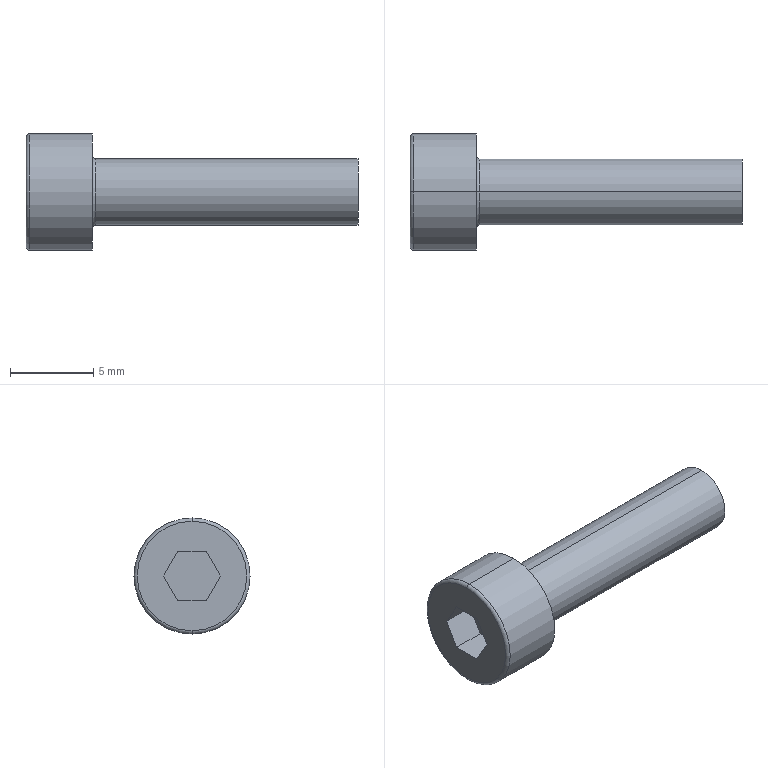Part | SolidWorks | features BlendCut 1, Cut 1, Fillet 1, LPattern 1, RevCut 1, Revolution 1 | 1 solid | 18 faces | box 20 x 7 x 7 mm | volume 339.552 mm3 | plane 10 | torus 4 | cylinder 4 | commonest cylinder face diameters 4 x2 7 x2
STEP:
#1=CARTESIAN_POINT('',(0.2,0.,-3.5));
#2=VERTEX_POINT('',#1);
#3=CARTESIAN_POINT('',(0.2,0.,3.5));
#4=VERTEX_POINT('',#3);
#5=CARTESIAN_POINT('',(0.2,0.,0.));
#6=DIRECTION('',(1.,0.,0.));
#7=DIRECTION('',(0.,0.,1.));
#8=AXIS2_PLACEMENT_3D('',#5,#6,#7);
#9=CIRCLE('',#8,3.5);
#10=EDGE_CURVE('',#2,#4,#9,.T.);
#11=ORIENTED_EDGE('',*,*,#10,.F.);
#12=CARTESIAN_POINT('',(0.,0.,-3.3));
#13=VERTEX_POINT('',#12);
#14=CARTESIAN_POINT('',(0.2,0.,-3.3));
#15=DIRECTION('',(0.,1.,0.));
#16=DIRECTION('',(0.,0.,1.));
#17=AXIS2_PLACEMENT_3D('',#14,#15,#16);
#18=CIRCLE('',#17,0.2);
#19=EDGE_CURVE('',#2,#13,#18,.T.);
#20=ORIENTED_EDGE('',*,*,#19,.T.);
#21=CARTESIAN_POINT('',(0.,0.,3.3));
#22=VERTEX_POINT('',#21);
#23=CARTESIAN_POINT('',(0.,0.,0.));
#24=DIRECTION('',(-1.,0.,0.));
#25=DIRECTION('',(0.,0.,1.));
#26=AXIS2_PLACEMENT_3D('',#23,#24,#25);
#27=CIRCLE('',#26,3.3);
#28=EDGE_CURVE('',#22,#13,#27,.T.);
#29=ORIENTED_EDGE('',*,*,#28,.F.);
#30=CARTESIAN_POINT('',(0.2,0.,3.3));
#31=DIRECTION('',(0.,-1.,0.));
#32=DIRECTION('',(0.,0.,-1.));
#33=AXIS2_PLACEMENT_3D('',#30,#31,#32);
#34=CIRCLE('',#33,0.2);
#35=EDGE_CURVE('',#4,#22,#34,.T.);
#36=ORIENTED_EDGE('',*,*,#35,.F.);
#37=EDGE_LOOP('',(#11,#20,#29,#36));
#38=FACE_OUTER_BOUND('',#37,.T.);
#39=CARTESIAN_POINT('',(0.2,0.,0.));
#40=DIRECTION('',(-1.,0.,0.));
#41=DIRECTION('',(0.,0.,1.));
#42=AXIS2_PLACEMENT_3D('',#39,#40,#41);
#43=TOROIDAL_SURFACE('',#42,3.3,0.2);
#44=ADVANCED_FACE('',(#38),#43,.T.);
#45=CARTESIAN_POINT('',(4.2,0.,-2.));
#46=VERTEX_POINT('',#45);
#47=CARTESIAN_POINT('',(4.2,0.,2.));
#48=VERTEX_POINT('',#47);
#49=CARTESIAN_POINT('',(4.2,0.,0.));
#50=DIRECTION('',(1.,0.,0.));
#51=DIRECTION('',(0.,0.,-1.));
#52=AXIS2_PLACEMENT_3D('',#49,#50,#51);
#53=CIRCLE('',#52,2.);
#54=EDGE_CURVE('',#46,#48,#53,.T.);
#55=ORIENTED_EDGE('',*,*,#54,.T.);
#56=CARTESIAN_POINT('',(20.,0.,2.));
#57=VERTEX_POINT('',#56);
#58=CARTESIAN_POINT('',(0.,0.,2.));
#59=DIRECTION('',(1.,0.,0.));
#60=VECTOR('',#59,1000.);
#61=LINE('',#58,#60);
#62=EDGE_CURVE('',#48,#57,#61,.T.);
#63=ORIENTED_EDGE('',*,*,#62,.T.);
#64=CARTESIAN_POINT('',(20.,0.,-2.));
#65=VERTEX_POINT('',#64);
#66=CARTESIAN_POINT('',(20.,0.,0.));
#67=DIRECTION('',(1.,0.,0.));
#68=DIRECTION('',(0.,0.,-1.));
#69=AXIS2_PLACEMENT_3D('',#66,#67,#68);
#70=CIRCLE('',#69,2.);
#71=EDGE_CURVE('',#65,#57,#70,.T.);
#72=ORIENTED_EDGE('',*,*,#71,.F.);
#73=CARTESIAN_POINT('',(0.,0.,-2.));
#74=DIRECTION('',(1.,0.,0.));
#75=VECTOR('',#74,1000.);
#76=LINE('',#73,#75);
#77=EDGE_CURVE('',#46,#65,#76,.T.);
#78=ORIENTED_EDGE('',*,*,#77,.F.);
#79=EDGE_LOOP('',(#55,#63,#72,#78));
#80=FACE_OUTER_BOUND('',#79,.T.);
#81=CARTESIAN_POINT('',(0.,0.,0.));
#82=DIRECTION('',(1.,0.,0.));
#83=DIRECTION('',(0.,0.,-1.));
#84=AXIS2_PLACEMENT_3D('',#81,#82,#83);
#85=CYLINDRICAL_SURFACE('',#84,2.);
#86=ADVANCED_FACE('',(#80),#85,.T.);
#87=CARTESIAN_POINT('',(4.2,0.,0.));
#88=DIRECTION('',(1.,0.,0.));
#89=DIRECTION('',(0.,0.,-1.));
#90=AXIS2_PLACEMENT_3D('',#87,#88,#89);
#91=CIRCLE('',#90,2.);
#92=EDGE_CURVE('',#48,#46,#91,.T.);
#93=ORIENTED_EDGE('',*,*,#92,.F.);
#94=CARTESIAN_POINT('',(4.,0.,2.2));
#95=VERTEX_POINT('',#94);
#96=CARTESIAN_POINT('',(4.2,0.,2.2));
#97=DIRECTION('',(0.,1.,0.));
#98=DIRECTION('',(0.,0.,1.));
#99=AXIS2_PLACEMENT_3D('',#96,#97,#98);
#100=CIRCLE('',#99,0.2);
#101=EDGE_CURVE('',#48,#95,#100,.T.);
#102=ORIENTED_EDGE('',*,*,#101,.T.);
#103=CARTESIAN_POINT('',(4.,0.,-2.2));
#104=VERTEX_POINT('',#103);
#105=CARTESIAN_POINT('',(4.,0.,0.));
#106=DIRECTION('',(1.,0.,0.));
#107=DIRECTION('',(0.,0.,-1.));
#108=AXIS2_PLACEMENT_3D('',#105,#106,#107);
#109=CIRCLE('',#108,2.2);
#110=EDGE_CURVE('',#95,#104,#109,.T.);
#111=ORIENTED_EDGE('',*,*,#110,.T.);
#112=CARTESIAN_POINT('',(4.2,0.,-2.2));
#113=DIRECTION('',(0.,-1.,0.));
#114=DIRECTION('',(0.,0.,-1.));
#115=AXIS2_PLACEMENT_3D('',#112,#113,#114);
#116=CIRCLE('',#115,0.2);
#117=EDGE_CURVE('',#46,#104,#116,.T.);
#118=ORIENTED_EDGE('',*,*,#117,.F.);
#119=EDGE_LOOP('',(#93,#102,#111,#118));
#120=FACE_OUTER_BOUND('',#119,.T.);
#121=CARTESIAN_POINT('',(4.2,0.,0.));
#122=DIRECTION('',(1.,0.,0.));
#123=DIRECTION('',(0.,0.,-1.));
#124=AXIS2_PLACEMENT_3D('',#121,#122,#123);
#125=TOROIDAL_SURFACE('',#124,2.2,0.2);
#126=ADVANCED_FACE('',(#120),#125,.F.);
#127=ORIENTED_EDGE('',*,*,#10,.T.);
#128=CARTESIAN_POINT('',(4.,0.,3.5));
#129=VERTEX_POINT('',#128);
#130=CARTESIAN_POINT('',(0.,0.,3.5));
#131=DIRECTION('',(1.,0.,0.));
#132=VECTOR('',#131,1000.);
#133=LINE('',#130,#132);
#134=EDGE_CURVE('',#4,#129,#133,.T.);
#135=ORIENTED_EDGE('',*,*,#134,.T.);
#136=CARTESIAN_POINT('',(4.,0.,-3.5));
#137=VERTEX_POINT('',#136);
#138=CARTESIAN_POINT('',(4.,0.,0.));
#139=DIRECTION('',(1.,0.,0.));
#140=DIRECTION('',(0.,0.,-1.));
#141=AXIS2_PLACEMENT_3D('',#138,#139,#140);
#142=CIRCLE('',#141,3.5);
#143=EDGE_CURVE('',#137,#129,#142,.T.);
#144=ORIENTED_EDGE('',*,*,#143,.F.);
#145=CARTESIAN_POINT('',(0.,0.,-3.5));
#146=DIRECTION('',(1.,0.,0.));
#147=VECTOR('',#146,1000.);
#148=LINE('',#145,#147);
#149=EDGE_CURVE('',#2,#137,#148,.T.);
#150=ORIENTED_EDGE('',*,*,#149,.F.);
#151=EDGE_LOOP('',(#127,#135,#144,#150));
#152=FACE_OUTER_BOUND('',#151,.T.);
#153=CARTESIAN_POINT('',(0.,0.,0.));
#154=DIRECTION('',(1.,0.,0.));
#155=DIRECTION('',(0.,0.,-1.));
#156=AXIS2_PLACEMENT_3D('',#153,#154,#155);
#157=CYLINDRICAL_SURFACE('',#156,3.5);
#158=ADVANCED_FACE('',(#152),#157,.T.);
#159=ORIENTED_EDGE('',*,*,#28,.T.);
#160=CARTESIAN_POINT('',(0.,0.,0.));
#161=DIRECTION('',(-1.,0.,0.));
#162=DIRECTION('',(0.,0.,1.));
#163=AXIS2_PLACEMENT_3D('',#160,#161,#162);
#164=CIRCLE('',#163,3.3);
#165=EDGE_CURVE('',#13,#22,#164,.T.);
#166=ORIENTED_EDGE('',*,*,#165,.T.);
#167=EDGE_LOOP('',(#159,#166));
#168=FACE_OUTER_BOUND('',#167,.T.);
#169=CARTESIAN_POINT('',(0.,-1.72,0.));
#170=VERTEX_POINT('',#169);
#171=CARTESIAN_POINT('',(0.,-0.86,1.49));
#172=VERTEX_POINT('',#171);
#173=CARTESIAN_POINT('',(0.,-1.72,0.));
#174=DIRECTION('',(0.,0.5,0.866));
#175=VECTOR('',#174,1000.);
#176=LINE('',#173,#175);
#177=EDGE_CURVE('',#170,#172,#176,.T.);
#178=ORIENTED_EDGE('',*,*,#177,.F.);
#179=CARTESIAN_POINT('',(0.,-0.86,-1.49));
#180=VERTEX_POINT('',#179);
#181=CARTESIAN_POINT('',(0.,-0.86,-1.49));
#182=DIRECTION('',(0.,-0.5,0.866));
#183=VECTOR('',#182,1000.);
#184=LINE('',#181,#183);
#185=EDGE_CURVE('',#180,#170,#184,.T.);
#186=ORIENTED_EDGE('',*,*,#185,.F.);
#187=CARTESIAN_POINT('',(0.,0.86,-1.49));
#188=VERTEX_POINT('',#187);
#189=CARTESIAN_POINT('',(0.,0.86,-1.49));
#190=DIRECTION('',(0.,-1.,0.));
#191=VECTOR('',#190,1000.);
#192=LINE('',#189,#191);
#193=EDGE_CURVE('',#188,#180,#192,.T.);
#194=ORIENTED_EDGE('',*,*,#193,.F.);
#195=CARTESIAN_POINT('',(0.,1.72,0.));
#196=VERTEX_POINT('',#195);
#197=CARTESIAN_POINT('',(0.,1.72,0.));
#198=DIRECTION('',(0.,-0.5,-0.866));
#199=VECTOR('',#198,1000.);
#200=LINE('',#197,#199);
#201=EDGE_CURVE('',#196,#188,#200,.T.);
#202=ORIENTED_EDGE('',*,*,#201,.F.);
#203=CARTESIAN_POINT('',(0.,0.86,1.49));
#204=VERTEX_POINT('',#203);
#205=CARTESIAN_POINT('',(0.,0.86,1.49));
#206=DIRECTION('',(0.,0.5,-0.866));
#207=VECTOR('',#206,1000.);
#208=LINE('',#205,#207);
#209=EDGE_CURVE('',#204,#196,#208,.T.);
#210=ORIENTED_EDGE('',*,*,#209,.F.);
#211=CARTESIAN_POINT('',(0.,-0.86,1.49));
#212=DIRECTION('',(0.,1.,0.));
#213=VECTOR('',#212,1000.);
#214=LINE('',#211,#213);
#215=EDGE_CURVE('',#172,#204,#214,.T.);
#216=ORIENTED_EDGE('',*,*,#215,.F.);
#217=EDGE_LOOP('',(#178,#186,#194,#202,#210,#216));
#218=FACE_BOUND('',#217,.T.);
#219=CARTESIAN_POINT('',(0.,0.,0.));
#220=DIRECTION('',(-1.,0.,0.));
#221=DIRECTION('',(0.,0.,1.));
#222=AXIS2_PLACEMENT_3D('',#219,#220,#221);
#223=PLANE('',#222);
#224=ADVANCED_FACE('',(#168,#218),#223,.T.);
#225=ORIENTED_EDGE('',*,*,#134,.F.);
#226=CARTESIAN_POINT('',(0.2,0.,0.));
#227=DIRECTION('',(1.,0.,0.));
#228=DIRECTION('',(0.,0.,1.));
#229=AXIS2_PLACEMENT_3D('',#226,#227,#228);
#230=CIRCLE('',#229,3.5);
#231=EDGE_CURVE('',#4,#2,#230,.T.);
#232=ORIENTED_EDGE('',*,*,#231,.T.);
#233=ORIENTED_EDGE('',*,*,#149,.T.);
#234=CARTESIAN_POINT('',(4.,0.,0.));
#235=DIRECTION('',(1.,0.,0.));
#236=DIRECTION('',(0.,0.,-1.));
#237=AXIS2_PLACEMENT_3D('',#234,#235,#236);
#238=CIRCLE('',#237,3.5);
#239=EDGE_CURVE('',#129,#137,#238,.T.);
#240=ORIENTED_EDGE('',*,*,#239,.F.);
#241=EDGE_LOOP('',(#225,#232,#233,#240));
#242=FACE_OUTER_BOUND('',#241,.T.);
#243=CARTESIAN_POINT('',(0.,0.,0.));
#244=DIRECTION('',(1.,0.,0.));
#245=DIRECTION('',(0.,0.,-1.));
#246=AXIS2_PLACEMENT_3D('',#243,#244,#245);
#247=CYLINDRICAL_SURFACE('',#246,3.5);
#248=ADVANCED_FACE('',(#242),#247,.T.);
#249=ORIENTED_EDGE('',*,*,#143,.T.);
#250=ORIENTED_EDGE('',*,*,#239,.T.);
#251=EDGE_LOOP('',(#249,#250));
#252=FACE_OUTER_BOUND('',#251,.T.);
#253=CARTESIAN_POINT('',(4.,0.,0.));
#254=DIRECTION('',(1.,0.,0.));
#255=DIRECTION('',(0.,0.,-1.));
#256=AXIS2_PLACEMENT_3D('',#253,#254,#255);
#257=CIRCLE('',#256,2.2);
#258=EDGE_CURVE('',#104,#95,#257,.T.);
#259=ORIENTED_EDGE('',*,*,#258,.F.);
#260=ORIENTED_EDGE('',*,*,#110,.F.);
#261=EDGE_LOOP('',(#259,#260));
#262=FACE_BOUND('',#261,.T.);
#263=CARTESIAN_POINT('',(4.,3.5,0.));
#264=DIRECTION('',(1.,0.,0.));
#265=DIRECTION('',(0.,0.,-1.));
#266=AXIS2_PLACEMENT_3D('',#263,#264,#265);
#267=PLANE('',#266);
#268=ADVANCED_FACE('',(#252,#262),#267,.T.);
#269=ORIENTED_EDGE('',*,*,#101,.F.);
#270=ORIENTED_EDGE('',*,*,#54,.F.);
#271=ORIENTED_EDGE('',*,*,#117,.T.);
#272=ORIENTED_EDGE('',*,*,#258,.T.);
#273=EDGE_LOOP('',(#269,#270,#271,#272));
#274=FACE_OUTER_BOUND('',#273,.T.);
#275=CARTESIAN_POINT('',(4.2,0.,0.));
#276=DIRECTION('',(1.,0.,0.));
#277=DIRECTION('',(0.,0.,-1.));
#278=AXIS2_PLACEMENT_3D('',#275,#276,#277);
#279=TOROIDAL_SURFACE('',#278,2.2,0.2);
#280=ADVANCED_FACE('',(#274),#279,.F.);
#281=ORIENTED_EDGE('',*,*,#62,.F.);
#282=ORIENTED_EDGE('',*,*,#92,.T.);
#283=ORIENTED_EDGE('',*,*,#77,.T.);
#284=CARTESIAN_POINT('',(20.,0.,0.));
#285=DIRECTION('',(1.,0.,0.));
#286=DIRECTION('',(0.,0.,-1.));
#287=AXIS2_PLACEMENT_3D('',#284,#285,#286);
#288=CIRCLE('',#287,2.);
#289=EDGE_CURVE('',#57,#65,#288,.T.);
#290=ORIENTED_EDGE('',*,*,#289,.F.);
#291=EDGE_LOOP('',(#281,#282,#283,#290));
#292=FACE_OUTER_BOUND('',#291,.T.);
#293=CARTESIAN_POINT('',(0.,0.,0.));
#294=DIRECTION('',(1.,0.,0.));
#295=DIRECTION('',(0.,0.,-1.));
#296=AXIS2_PLACEMENT_3D('',#293,#294,#295);
#297=CYLINDRICAL_SURFACE('',#296,2.);
#298=ADVANCED_FACE('',(#292),#297,.T.);
#299=ORIENTED_EDGE('',*,*,#71,.T.);
#300=ORIENTED_EDGE('',*,*,#289,.T.);
#301=EDGE_LOOP('',(#299,#300));
#302=FACE_OUTER_BOUND('',#301,.T.);
#303=CARTESIAN_POINT('',(20.,2.,0.));
#304=DIRECTION('',(1.,0.,0.));
#305=DIRECTION('',(0.,0.,-1.));
#306=AXIS2_PLACEMENT_3D('',#303,#304,#305);
#307=PLANE('',#306);
#308=ADVANCED_FACE('',(#302),#307,.T.);
#309=ORIENTED_EDGE('',*,*,#177,.T.);
#310=CARTESIAN_POINT('',(2.,-0.86,1.49));
#311=VERTEX_POINT('',#310);
#312=CARTESIAN_POINT('',(2.,-0.86,1.49));
#313=DIRECTION('',(-1.,0.,0.));
#314=VECTOR('',#313,1000.);
#315=LINE('',#312,#314);
#316=EDGE_CURVE('',#311,#172,#315,.T.);
#317=ORIENTED_EDGE('',*,*,#316,.F.);
#318=CARTESIAN_POINT('',(2.,-1.72,0.));
#319=VERTEX_POINT('',#318);
#320=CARTESIAN_POINT('',(2.,-1.72,0.));
#321=DIRECTION('',(0.,0.5,0.866));
#322=VECTOR('',#321,1000.);
#323=LINE('',#320,#322);
#324=EDGE_CURVE('',#319,#311,#323,.T.);
#325=ORIENTED_EDGE('',*,*,#324,.F.);
#326=CARTESIAN_POINT('',(2.,-1.72,0.));
#327=DIRECTION('',(-1.,0.,0.));
#328=VECTOR('',#327,1000.);
#329=LINE('',#326,#328);
#330=EDGE_CURVE('',#319,#170,#329,.T.);
#331=ORIENTED_EDGE('',*,*,#330,.T.);
#332=EDGE_LOOP('',(#309,#317,#325,#331));
#333=FACE_OUTER_BOUND('',#332,.T.);
#334=CARTESIAN_POINT('',(2.,-1.72,0.));
#335=DIRECTION('',(0.,-0.866,0.5));
#336=DIRECTION('',(0.,-0.5,-0.866));
#337=AXIS2_PLACEMENT_3D('',#334,#335,#336);
#338=PLANE('',#337);
#339=ADVANCED_FACE('',(#333),#338,.F.);
#340=ORIENTED_EDGE('',*,*,#185,.T.);
#341=ORIENTED_EDGE('',*,*,#330,.F.);
#342=CARTESIAN_POINT('',(2.,-0.86,-1.49));
#343=VERTEX_POINT('',#342);
#344=CARTESIAN_POINT('',(2.,-0.86,-1.49));
#345=DIRECTION('',(0.,-0.5,0.866));
#346=VECTOR('',#345,1000.);
#347=LINE('',#344,#346);
#348=EDGE_CURVE('',#343,#319,#347,.T.);
#349=ORIENTED_EDGE('',*,*,#348,.F.);
#350=CARTESIAN_POINT('',(2.,-0.86,-1.49));
#351=DIRECTION('',(-1.,0.,0.));
#352=VECTOR('',#351,1000.);
#353=LINE('',#350,#352);
#354=EDGE_CURVE('',#343,#180,#353,.T.);
#355=ORIENTED_EDGE('',*,*,#354,.T.);
#356=EDGE_LOOP('',(#340,#341,#349,#355));
#357=FACE_OUTER_BOUND('',#356,.T.);
#358=CARTESIAN_POINT('',(2.,-0.86,-1.49));
#359=DIRECTION('',(0.,-0.866,-0.5));
#360=DIRECTION('',(0.,0.5,-0.866));
#361=AXIS2_PLACEMENT_3D('',#358,#359,#360);
#362=PLANE('',#361);
#363=ADVANCED_FACE('',(#357),#362,.F.);
#364=ORIENTED_EDGE('',*,*,#193,.T.);
#365=ORIENTED_EDGE('',*,*,#354,.F.);
#366=CARTESIAN_POINT('',(2.,0.86,-1.49));
#367=VERTEX_POINT('',#366);
#368=CARTESIAN_POINT('',(2.,0.86,-1.49));
#369=DIRECTION('',(0.,-1.,0.));
#370=VECTOR('',#369,1000.);
#371=LINE('',#368,#370);
#372=EDGE_CURVE('',#367,#343,#371,.T.);
#373=ORIENTED_EDGE('',*,*,#372,.F.);
#374=CARTESIAN_POINT('',(2.,0.86,-1.49));
#375=DIRECTION('',(-1.,0.,0.));
#376=VECTOR('',#375,1000.);
#377=LINE('',#374,#376);
#378=EDGE_CURVE('',#367,#188,#377,.T.);
#379=ORIENTED_EDGE('',*,*,#378,.T.);
#380=EDGE_LOOP('',(#364,#365,#373,#379));
#381=FACE_OUTER_BOUND('',#380,.T.);
#382=CARTESIAN_POINT('',(2.,0.86,-1.49));
#383=DIRECTION('',(0.,0.,-1.));
#384=DIRECTION('',(0.,1.,0.));
#385=AXIS2_PLACEMENT_3D('',#382,#383,#384);
#386=PLANE('',#385);
#387=ADVANCED_FACE('',(#381),#386,.F.);
#388=ORIENTED_EDGE('',*,*,#201,.T.);
#389=ORIENTED_EDGE('',*,*,#378,.F.);
#390=CARTESIAN_POINT('',(2.,1.72,0.));
#391=VERTEX_POINT('',#390);
#392=CARTESIAN_POINT('',(2.,1.72,0.));
#393=DIRECTION('',(0.,-0.5,-0.866));
#394=VECTOR('',#393,1000.);
#395=LINE('',#392,#394);
#396=EDGE_CURVE('',#391,#367,#395,.T.);
#397=ORIENTED_EDGE('',*,*,#396,.F.);
#398=CARTESIAN_POINT('',(2.,1.72,0.));
#399=DIRECTION('',(-1.,0.,0.));
#400=VECTOR('',#399,1000.);
#401=LINE('',#398,#400);
#402=EDGE_CURVE('',#391,#196,#401,.T.);
#403=ORIENTED_EDGE('',*,*,#402,.T.);
#404=EDGE_LOOP('',(#388,#389,#397,#403));
#405=FACE_OUTER_BOUND('',#404,.T.);
#406=CARTESIAN_POINT('',(2.,1.72,0.));
#407=DIRECTION('',(0.,0.866,-0.5));
#408=DIRECTION('',(0.,0.5,0.866));
#409=AXIS2_PLACEMENT_3D('',#406,#407,#408);
#410=PLANE('',#409);
#411=ADVANCED_FACE('',(#405),#410,.F.);
#412=ORIENTED_EDGE('',*,*,#209,.T.);
#413=ORIENTED_EDGE('',*,*,#402,.F.);
#414=CARTESIAN_POINT('',(2.,0.86,1.49));
#415=VERTEX_POINT('',#414);
#416=CARTESIAN_POINT('',(2.,0.86,1.49));
#417=DIRECTION('',(0.,0.5,-0.866));
#418=VECTOR('',#417,1000.);
#419=LINE('',#416,#418);
#420=EDGE_CURVE('',#415,#391,#419,.T.);
#421=ORIENTED_EDGE('',*,*,#420,.F.);
#422=CARTESIAN_POINT('',(2.,0.86,1.49));
#423=DIRECTION('',(-1.,0.,0.));
#424=VECTOR('',#423,1000.);
#425=LINE('',#422,#424);
#426=EDGE_CURVE('',#415,#204,#425,.T.);
#427=ORIENTED_EDGE('',*,*,#426,.T.);
#428=EDGE_LOOP('',(#412,#413,#421,#427));
#429=FACE_OUTER_BOUND('',#428,.T.);
#430=CARTESIAN_POINT('',(2.,0.86,1.49));
#431=DIRECTION('',(0.,0.866,0.5));
#432=DIRECTION('',(0.,-0.5,0.866));
#433=AXIS2_PLACEMENT_3D('',#430,#431,#432);
#434=PLANE('',#433);
#435=ADVANCED_FACE('',(#429),#434,.F.);
#436=ORIENTED_EDGE('',*,*,#215,.T.);
#437=ORIENTED_EDGE('',*,*,#426,.F.);
#438=CARTESIAN_POINT('',(2.,-0.86,1.49));
#439=DIRECTION('',(0.,1.,0.));
#440=VECTOR('',#439,1000.);
#441=LINE('',#438,#440);
#442=EDGE_CURVE('',#311,#415,#441,.T.);
#443=ORIENTED_EDGE('',*,*,#442,.F.);
#444=ORIENTED_EDGE('',*,*,#316,.T.);
#445=EDGE_LOOP('',(#436,#437,#443,#444));
#446=FACE_OUTER_BOUND('',#445,.T.);
#447=CARTESIAN_POINT('',(2.,-0.86,1.49));
#448=DIRECTION('',(0.,0.,1.));
#449=DIRECTION('',(0.,-1.,0.));
#450=AXIS2_PLACEMENT_3D('',#447,#448,#449);
#451=PLANE('',#450);
#452=ADVANCED_FACE('',(#446),#451,.F.);
#453=ORIENTED_EDGE('',*,*,#324,.T.);
#454=ORIENTED_EDGE('',*,*,#442,.T.);
#455=ORIENTED_EDGE('',*,*,#420,.T.);
#456=ORIENTED_EDGE('',*,*,#396,.T.);
#457=ORIENTED_EDGE('',*,*,#372,.T.);
#458=ORIENTED_EDGE('',*,*,#348,.T.);
#459=EDGE_LOOP('',(#453,#454,#455,#456,#457,#458));
#460=FACE_OUTER_BOUND('',#459,.T.);
#461=CARTESIAN_POINT('',(2.,-0.86,1.49));
#462=DIRECTION('',(-1.,0.,0.));
#463=DIRECTION('',(0.,0.,1.));
#464=AXIS2_PLACEMENT_3D('',#461,#462,#463);
#465=PLANE('',#464);
#466=ADVANCED_FACE('',(#460),#465,.T.);
#467=ORIENTED_EDGE('',*,*,#19,.F.);
#468=ORIENTED_EDGE('',*,*,#231,.F.);
#469=ORIENTED_EDGE('',*,*,#35,.T.);
#470=ORIENTED_EDGE('',*,*,#165,.F.);
#471=EDGE_LOOP('',(#467,#468,#469,#470));
#472=FACE_OUTER_BOUND('',#471,.T.);
#473=CARTESIAN_POINT('',(0.2,0.,0.));
#474=DIRECTION('',(-1.,0.,0.));
#475=DIRECTION('',(0.,0.,1.));
#476=AXIS2_PLACEMENT_3D('',#473,#474,#475);
#477=TOROIDAL_SURFACE('',#476,3.3,0.2);
#478=ADVANCED_FACE('',(#472),#477,.T.);
#479=CLOSED_SHELL('',(#44,#86,#126,#158,#224,#248,#268,#280,#298,#308,#339,#363,#387,#411,#435,#452,#466,#478));
#480=MANIFOLD_SOLID_BREP('',#479);
#481=CARTESIAN_POINT('',(0.,0.,0.));
#482=DIRECTION('',(0.,0.,1.));
#483=DIRECTION('',(1.,0.,0.));
#484=AXIS2_PLACEMENT_3D('',#481,#482,#483);
#485=(LENGTH_UNIT()NAMED_UNIT(*)SI_UNIT(.MILLI.,.METRE.));
#486=UNCERTAINTY_MEASURE_WITH_UNIT(LENGTH_MEASURE(0.00001),#485,'','');
#487=(NAMED_UNIT(*)PLANE_ANGLE_UNIT()SI_UNIT($,.RADIAN.));
#488=(NAMED_UNIT(*)SI_UNIT($,.STERADIAN.)SOLID_ANGLE_UNIT());
#489=(GEOMETRIC_REPRESENTATION_CONTEXT(3)GLOBAL_UNCERTAINTY_ASSIGNED_CONTEXT((#486))GLOBAL_UNIT_ASSIGNED_CONTEXT((#485,#487,#488))REPRESENTATION_CONTEXT('',''));
#490=ADVANCED_BREP_SHAPE_REPRESENTATION('',(#480,#484),#489);